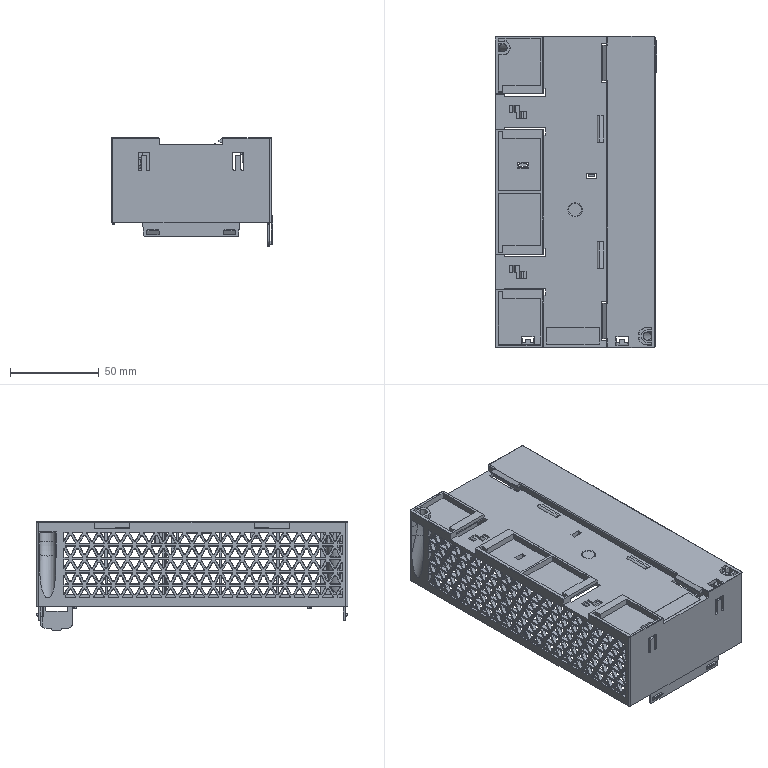Part | Creo | 1 solid | 4013 faces | volume 75306 mm3 | spline 1550 | plane 1364 | cone 823 | cylinder 242 | torus 20 | sphere 10 | other 4 | commonest cylinder face diameters 0.6 x85 0.4 x58 1 x41 2 x14 39.999 x8 5 x4